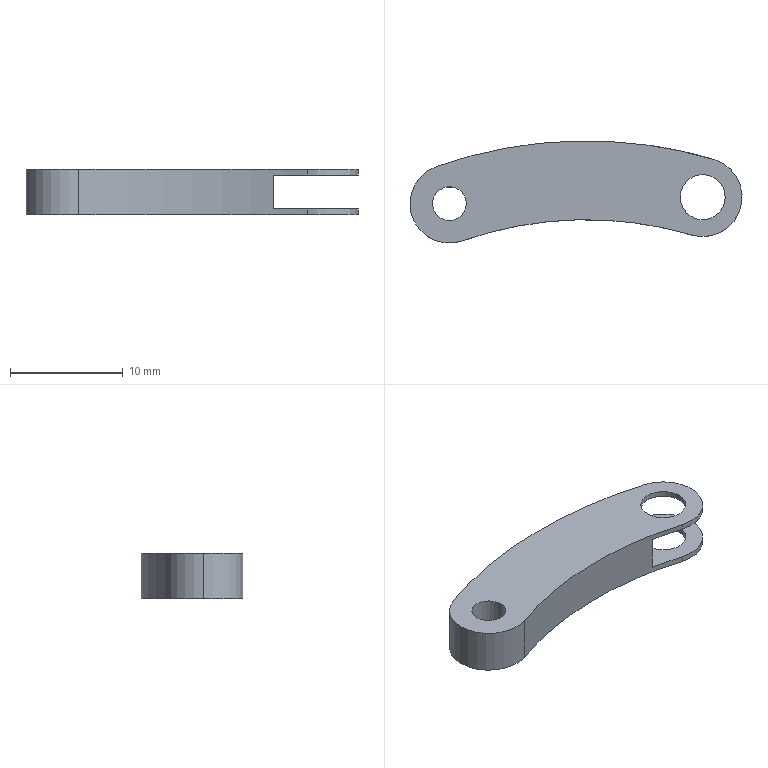Part | SolidWorks | features Extrusion 1, ICE 1, Scale 1 | 1 solid | 17 faces | box 29.5 x 9.079 x 4 mm | volume 609.677 mm3 | cylinder 12 | plane 5 | commonest cylinder face diameters 4 x4 7 x4 3 x2 66 x1 80 x1
STEP:
#1=CARTESIAN_POINT('',(-25.715,-3.325,4.));
#2=VERTEX_POINT('',#1);
#3=CARTESIAN_POINT('',(-22.715,-3.325,4.));
#4=VERTEX_POINT('',#3);
#5=CARTESIAN_POINT('',(-24.215,-3.325,4.));
#6=DIRECTION('',(0.,0.,1.));
#7=DIRECTION('',(1.,0.,0.));
#8=AXIS2_PLACEMENT_3D('',#5,#6,#7);
#9=CIRCLE('',#8,1.5);
#10=EDGE_CURVE('',#2,#4,#9,.T.);
#11=ORIENTED_EDGE('',*,*,#10,.T.);
#12=CARTESIAN_POINT('',(-22.715,-3.325,0.));
#13=VERTEX_POINT('',#12);
#14=CARTESIAN_POINT('',(-22.715,-3.325,4.));
#15=DIRECTION('',(0.,0.,-1.));
#16=VECTOR('',#15,1000.);
#17=LINE('',#14,#16);
#18=EDGE_CURVE('',#4,#13,#17,.T.);
#19=ORIENTED_EDGE('',*,*,#18,.T.);
#20=CARTESIAN_POINT('',(-25.715,-3.325,0.));
#21=VERTEX_POINT('',#20);
#22=CARTESIAN_POINT('',(-24.215,-3.325,0.));
#23=DIRECTION('',(0.,0.,1.));
#24=DIRECTION('',(1.,0.,0.));
#25=AXIS2_PLACEMENT_3D('',#22,#23,#24);
#26=CIRCLE('',#25,1.5);
#27=EDGE_CURVE('',#21,#13,#26,.T.);
#28=ORIENTED_EDGE('',*,*,#27,.F.);
#29=CARTESIAN_POINT('',(-25.715,-3.325,4.));
#30=DIRECTION('',(0.,0.,-1.));
#31=VECTOR('',#30,1000.);
#32=LINE('',#29,#31);
#33=EDGE_CURVE('',#2,#21,#32,.T.);
#34=ORIENTED_EDGE('',*,*,#33,.F.);
#35=EDGE_LOOP('',(#11,#19,#28,#34));
#36=FACE_OUTER_BOUND('',#35,.T.);
#37=CARTESIAN_POINT('',(-24.215,-3.325,4.));
#38=DIRECTION('',(0.,0.,-1.));
#39=DIRECTION('',(-1.,0.,0.));
#40=AXIS2_PLACEMENT_3D('',#37,#38,#39);
#41=CYLINDRICAL_SURFACE('',#40,1.5);
#42=ADVANCED_FACE('',(#36),#41,.F.);
#43=CARTESIAN_POINT('',(-27.715,-3.325,4.));
#44=VERTEX_POINT('',#43);
#45=CARTESIAN_POINT('',(-23.05,-6.626,4.));
#46=VERTEX_POINT('',#45);
#47=CARTESIAN_POINT('',(-24.215,-3.325,4.));
#48=DIRECTION('',(0.,0.,1.));
#49=DIRECTION('',(1.,0.,0.));
#50=AXIS2_PLACEMENT_3D('',#47,#48,#49);
#51=CIRCLE('',#50,3.5);
#52=EDGE_CURVE('',#44,#46,#51,.T.);
#53=ORIENTED_EDGE('',*,*,#52,.F.);
#54=CARTESIAN_POINT('',(-27.715,-3.325,0.));
#55=VERTEX_POINT('',#54);
#56=CARTESIAN_POINT('',(-27.715,-3.325,4.));
#57=DIRECTION('',(0.,0.,-1.));
#58=VECTOR('',#57,1000.);
#59=LINE('',#56,#58);
#60=EDGE_CURVE('',#44,#55,#59,.T.);
#61=ORIENTED_EDGE('',*,*,#60,.T.);
#62=CARTESIAN_POINT('',(-23.05,-6.626,0.));
#63=VERTEX_POINT('',#62);
#64=CARTESIAN_POINT('',(-24.215,-3.325,0.));
#65=DIRECTION('',(0.,0.,1.));
#66=DIRECTION('',(1.,0.,0.));
#67=AXIS2_PLACEMENT_3D('',#64,#65,#66);
#68=CIRCLE('',#67,3.5);
#69=EDGE_CURVE('',#55,#63,#68,.T.);
#70=ORIENTED_EDGE('',*,*,#69,.T.);
#71=CARTESIAN_POINT('',(-23.05,-6.626,4.));
#72=DIRECTION('',(0.,0.,-1.));
#73=VECTOR('',#72,1000.);
#74=LINE('',#71,#73);
#75=EDGE_CURVE('',#46,#63,#74,.T.);
#76=ORIENTED_EDGE('',*,*,#75,.F.);
#77=EDGE_LOOP('',(#53,#61,#70,#76));
#78=FACE_OUTER_BOUND('',#77,.T.);
#79=CARTESIAN_POINT('',(-24.215,-3.325,4.));
#80=DIRECTION('',(0.,0.,-1.));
#81=DIRECTION('',(-1.,0.,0.));
#82=AXIS2_PLACEMENT_3D('',#79,#80,#81);
#83=CYLINDRICAL_SURFACE('',#82,3.5);
#84=ADVANCED_FACE('',(#78),#83,.T.);
#85=CARTESIAN_POINT('',(-3.715,-2.747,4.));
#86=VERTEX_POINT('',#85);
#87=CARTESIAN_POINT('',(0.2854,-2.747,4.));
#88=VERTEX_POINT('',#87);
#89=CARTESIAN_POINT('',(-1.715,-2.747,4.));
#90=DIRECTION('',(0.,0.,1.));
#91=DIRECTION('',(1.,0.,0.));
#92=AXIS2_PLACEMENT_3D('',#89,#90,#91);
#93=CIRCLE('',#92,2.);
#94=EDGE_CURVE('',#86,#88,#93,.T.);
#95=ORIENTED_EDGE('',*,*,#94,.T.);
#96=CARTESIAN_POINT('',(0.2854,-2.747,3.5));
#97=VERTEX_POINT('',#96);
#98=CARTESIAN_POINT('',(0.2854,-2.747,4.));
#99=DIRECTION('',(0.,0.,-1.));
#100=VECTOR('',#99,1000.);
#101=LINE('',#98,#100);
#102=EDGE_CURVE('',#88,#97,#101,.T.);
#103=ORIENTED_EDGE('',*,*,#102,.T.);
#104=CARTESIAN_POINT('',(-3.715,-2.747,3.5));
#105=VERTEX_POINT('',#104);
#106=CARTESIAN_POINT('',(-1.715,-2.747,3.5));
#107=DIRECTION('',(0.,0.,-1.));
#108=DIRECTION('',(-1.,0.,0.));
#109=AXIS2_PLACEMENT_3D('',#106,#107,#108);
#110=CIRCLE('',#109,2.);
#111=EDGE_CURVE('',#97,#105,#110,.T.);
#112=ORIENTED_EDGE('',*,*,#111,.T.);
#113=CARTESIAN_POINT('',(-3.715,-2.747,4.));
#114=DIRECTION('',(0.,0.,-1.));
#115=VECTOR('',#114,1000.);
#116=LINE('',#113,#115);
#117=EDGE_CURVE('',#86,#105,#116,.T.);
#118=ORIENTED_EDGE('',*,*,#117,.F.);
#119=EDGE_LOOP('',(#95,#103,#112,#118));
#120=FACE_OUTER_BOUND('',#119,.T.);
#121=CARTESIAN_POINT('',(-1.715,-2.747,4.));
#122=DIRECTION('',(0.,0.,-1.));
#123=DIRECTION('',(-1.,0.,0.));
#124=AXIS2_PLACEMENT_3D('',#121,#122,#123);
#125=CYLINDRICAL_SURFACE('',#124,2.);
#126=ADVANCED_FACE('',(#120),#125,.F.);
#127=CARTESIAN_POINT('',(-3.715,-2.747,0.5));
#128=VERTEX_POINT('',#127);
#129=CARTESIAN_POINT('',(0.2854,-2.747,0.5));
#130=VERTEX_POINT('',#129);
#131=CARTESIAN_POINT('',(-1.715,-2.747,0.5));
#132=DIRECTION('',(0.,0.,1.));
#133=DIRECTION('',(1.,0.,0.));
#134=AXIS2_PLACEMENT_3D('',#131,#132,#133);
#135=CIRCLE('',#134,2.);
#136=EDGE_CURVE('',#128,#130,#135,.T.);
#137=ORIENTED_EDGE('',*,*,#136,.T.);
#138=CARTESIAN_POINT('',(0.2854,-2.747,0.));
#139=VERTEX_POINT('',#138);
#140=CARTESIAN_POINT('',(0.2854,-2.747,4.));
#141=DIRECTION('',(0.,0.,-1.));
#142=VECTOR('',#141,1000.);
#143=LINE('',#140,#142);
#144=EDGE_CURVE('',#130,#139,#143,.T.);
#145=ORIENTED_EDGE('',*,*,#144,.T.);
#146=CARTESIAN_POINT('',(-3.715,-2.747,0.));
#147=VERTEX_POINT('',#146);
#148=CARTESIAN_POINT('',(-1.715,-2.747,0.));
#149=DIRECTION('',(0.,0.,1.));
#150=DIRECTION('',(1.,0.,0.));
#151=AXIS2_PLACEMENT_3D('',#148,#149,#150);
#152=CIRCLE('',#151,2.);
#153=EDGE_CURVE('',#147,#139,#152,.T.);
#154=ORIENTED_EDGE('',*,*,#153,.F.);
#155=CARTESIAN_POINT('',(-3.715,-2.747,4.));
#156=DIRECTION('',(0.,0.,-1.));
#157=VECTOR('',#156,1000.);
#158=LINE('',#155,#157);
#159=EDGE_CURVE('',#128,#147,#158,.T.);
#160=ORIENTED_EDGE('',*,*,#159,.F.);
#161=EDGE_LOOP('',(#137,#145,#154,#160));
#162=FACE_OUTER_BOUND('',#161,.T.);
#163=CARTESIAN_POINT('',(-1.715,-2.747,4.));
#164=DIRECTION('',(0.,0.,-1.));
#165=DIRECTION('',(-1.,0.,0.));
#166=AXIS2_PLACEMENT_3D('',#163,#164,#165);
#167=CYLINDRICAL_SURFACE('',#166,2.);
#168=ADVANCED_FACE('',(#162),#167,.F.);
#169=CARTESIAN_POINT('',(-5.715,-5.364,0.5));
#170=VERTEX_POINT('',#169);
#171=CARTESIAN_POINT('',(-2.708,-6.103,0.5));
#172=VERTEX_POINT('',#171);
#173=CARTESIAN_POINT('',(-12.072,-37.746,0.5));
#174=DIRECTION('',(0.,0.,-1.));
#175=DIRECTION('',(1.,0.,0.));
#176=AXIS2_PLACEMENT_3D('',#173,#174,#175);
#177=CIRCLE('',#176,33.);
#178=EDGE_CURVE('',#170,#172,#177,.T.);
#179=ORIENTED_EDGE('',*,*,#178,.F.);
#180=CARTESIAN_POINT('',(-5.715,-5.364,3.5));
#181=VERTEX_POINT('',#180);
#182=CARTESIAN_POINT('',(-5.715,-5.364,4.));
#183=DIRECTION('',(0.,0.,-1.));
#184=VECTOR('',#183,1000.);
#185=LINE('',#182,#184);
#186=EDGE_CURVE('',#181,#170,#185,.T.);
#187=ORIENTED_EDGE('',*,*,#186,.F.);
#188=CARTESIAN_POINT('',(-2.708,-6.103,3.5));
#189=VERTEX_POINT('',#188);
#190=CARTESIAN_POINT('',(-12.072,-37.746,3.5));
#191=DIRECTION('',(0.,0.,1.));
#192=DIRECTION('',(-1.,0.,0.));
#193=AXIS2_PLACEMENT_3D('',#190,#191,#192);
#194=CIRCLE('',#193,33.);
#195=EDGE_CURVE('',#189,#181,#194,.T.);
#196=ORIENTED_EDGE('',*,*,#195,.F.);
#197=CARTESIAN_POINT('',(-2.708,-6.103,4.));
#198=VERTEX_POINT('',#197);
#199=CARTESIAN_POINT('',(-2.708,-6.103,4.));
#200=DIRECTION('',(0.,0.,-1.));
#201=VECTOR('',#200,1000.);
#202=LINE('',#199,#201);
#203=EDGE_CURVE('',#198,#189,#202,.T.);
#204=ORIENTED_EDGE('',*,*,#203,.F.);
#205=CARTESIAN_POINT('',(-12.072,-37.746,4.));
#206=DIRECTION('',(0.,0.,-1.));
#207=DIRECTION('',(-1.,0.,0.));
#208=AXIS2_PLACEMENT_3D('',#205,#206,#207);
#209=CIRCLE('',#208,33.);
#210=EDGE_CURVE('',#46,#198,#209,.T.);
#211=ORIENTED_EDGE('',*,*,#210,.F.);
#212=ORIENTED_EDGE('',*,*,#75,.T.);
#213=CARTESIAN_POINT('',(-2.708,-6.103,0.));
#214=VERTEX_POINT('',#213);
#215=CARTESIAN_POINT('',(-12.072,-37.746,0.));
#216=DIRECTION('',(0.,0.,-1.));
#217=DIRECTION('',(-1.,0.,0.));
#218=AXIS2_PLACEMENT_3D('',#215,#216,#217);
#219=CIRCLE('',#218,33.);
#220=EDGE_CURVE('',#63,#214,#219,.T.);
#221=ORIENTED_EDGE('',*,*,#220,.T.);
#222=CARTESIAN_POINT('',(-2.708,-6.103,4.));
#223=DIRECTION('',(0.,0.,-1.));
#224=VECTOR('',#223,1000.);
#225=LINE('',#222,#224);
#226=EDGE_CURVE('',#172,#214,#225,.T.);
#227=ORIENTED_EDGE('',*,*,#226,.F.);
#228=EDGE_LOOP('',(#179,#187,#196,#204,#211,#212,#221,#227));
#229=FACE_OUTER_BOUND('',#228,.T.);
#230=CARTESIAN_POINT('',(-12.072,-37.746,4.));
#231=DIRECTION('',(0.,0.,-1.));
#232=DIRECTION('',(-1.,0.,0.));
#233=AXIS2_PLACEMENT_3D('',#230,#231,#232);
#234=CYLINDRICAL_SURFACE('',#233,33.);
#235=ADVANCED_FACE('',(#229),#234,.F.);
#236=CARTESIAN_POINT('',(-0.7214,0.6095,0.5));
#237=VERTEX_POINT('',#236);
#238=CARTESIAN_POINT('',(-1.715,-2.747,0.5));
#239=DIRECTION('',(0.,0.,1.));
#240=DIRECTION('',(1.,0.,0.));
#241=AXIS2_PLACEMENT_3D('',#238,#239,#240);
#242=CIRCLE('',#241,3.5);
#243=EDGE_CURVE('',#172,#237,#242,.T.);
#244=ORIENTED_EDGE('',*,*,#243,.F.);
#245=ORIENTED_EDGE('',*,*,#226,.T.);
#246=CARTESIAN_POINT('',(-0.7214,0.6095,0.));
#247=VERTEX_POINT('',#246);
#248=CARTESIAN_POINT('',(-1.715,-2.747,0.));
#249=DIRECTION('',(0.,0.,1.));
#250=DIRECTION('',(1.,0.,0.));
#251=AXIS2_PLACEMENT_3D('',#248,#249,#250);
#252=CIRCLE('',#251,3.5);
#253=EDGE_CURVE('',#214,#247,#252,.T.);
#254=ORIENTED_EDGE('',*,*,#253,.T.);
#255=CARTESIAN_POINT('',(-0.7214,0.6095,4.));
#256=DIRECTION('',(0.,0.,-1.));
#257=VECTOR('',#256,1000.);
#258=LINE('',#255,#257);
#259=EDGE_CURVE('',#237,#247,#258,.T.);
#260=ORIENTED_EDGE('',*,*,#259,.F.);
#261=EDGE_LOOP('',(#244,#245,#254,#260));
#262=FACE_OUTER_BOUND('',#261,.T.);
#263=CARTESIAN_POINT('',(-1.715,-2.747,4.));
#264=DIRECTION('',(0.,0.,-1.));
#265=DIRECTION('',(-1.,0.,0.));
#266=AXIS2_PLACEMENT_3D('',#263,#264,#265);
#267=CYLINDRICAL_SURFACE('',#266,3.5);
#268=ADVANCED_FACE('',(#262),#267,.T.);
#269=CARTESIAN_POINT('',(-0.7214,0.6095,3.5));
#270=VERTEX_POINT('',#269);
#271=CARTESIAN_POINT('',(-1.715,-2.747,3.5));
#272=DIRECTION('',(0.,0.,-1.));
#273=DIRECTION('',(-1.,0.,0.));
#274=AXIS2_PLACEMENT_3D('',#271,#272,#273);
#275=CIRCLE('',#274,3.5);
#276=EDGE_CURVE('',#270,#189,#275,.T.);
#277=ORIENTED_EDGE('',*,*,#276,.F.);
#278=CARTESIAN_POINT('',(-0.7214,0.6095,4.));
#279=VERTEX_POINT('',#278);
#280=CARTESIAN_POINT('',(-0.7214,0.6095,4.));
#281=DIRECTION('',(0.,0.,-1.));
#282=VECTOR('',#281,1000.);
#283=LINE('',#280,#282);
#284=EDGE_CURVE('',#279,#270,#283,.T.);
#285=ORIENTED_EDGE('',*,*,#284,.F.);
#286=CARTESIAN_POINT('',(-1.715,-2.747,4.));
#287=DIRECTION('',(0.,0.,1.));
#288=DIRECTION('',(1.,0.,0.));
#289=AXIS2_PLACEMENT_3D('',#286,#287,#288);
#290=CIRCLE('',#289,3.5);
#291=EDGE_CURVE('',#198,#279,#290,.T.);
#292=ORIENTED_EDGE('',*,*,#291,.F.);
#293=ORIENTED_EDGE('',*,*,#203,.T.);
#294=EDGE_LOOP('',(#277,#285,#292,#293));
#295=FACE_OUTER_BOUND('',#294,.T.);
#296=CARTESIAN_POINT('',(-1.715,-2.747,4.));
#297=DIRECTION('',(0.,0.,-1.));
#298=DIRECTION('',(-1.,0.,0.));
#299=AXIS2_PLACEMENT_3D('',#296,#297,#298);
#300=CYLINDRICAL_SURFACE('',#299,3.5);
#301=ADVANCED_FACE('',(#295),#300,.T.);
#302=CARTESIAN_POINT('',(-5.715,1.745,0.5));
#303=VERTEX_POINT('',#302);
#304=CARTESIAN_POINT('',(-12.072,-37.746,0.5));
#305=DIRECTION('',(0.,0.,1.));
#306=DIRECTION('',(1.,0.,0.));
#307=AXIS2_PLACEMENT_3D('',#304,#305,#306);
#308=CIRCLE('',#307,40.);
#309=EDGE_CURVE('',#237,#303,#308,.T.);
#310=ORIENTED_EDGE('',*,*,#309,.F.);
#311=ORIENTED_EDGE('',*,*,#259,.T.);
#312=CARTESIAN_POINT('',(-25.379,-0.0244,0.));
#313=VERTEX_POINT('',#312);
#314=CARTESIAN_POINT('',(-12.072,-37.746,0.));
#315=DIRECTION('',(0.,0.,1.));
#316=DIRECTION('',(-1.,0.,0.));
#317=AXIS2_PLACEMENT_3D('',#314,#315,#316);
#318=CIRCLE('',#317,40.);
#319=EDGE_CURVE('',#247,#313,#318,.T.);
#320=ORIENTED_EDGE('',*,*,#319,.T.);
#321=CARTESIAN_POINT('',(-25.379,-0.0244,4.));
#322=VERTEX_POINT('',#321);
#323=CARTESIAN_POINT('',(-25.379,-0.0244,4.));
#324=DIRECTION('',(0.,0.,-1.));
#325=VECTOR('',#324,1000.);
#326=LINE('',#323,#325);
#327=EDGE_CURVE('',#322,#313,#326,.T.);
#328=ORIENTED_EDGE('',*,*,#327,.F.);
#329=CARTESIAN_POINT('',(-12.072,-37.746,4.));
#330=DIRECTION('',(0.,0.,1.));
#331=DIRECTION('',(-1.,0.,0.));
#332=AXIS2_PLACEMENT_3D('',#329,#330,#331);
#333=CIRCLE('',#332,40.);
#334=EDGE_CURVE('',#279,#322,#333,.T.);
#335=ORIENTED_EDGE('',*,*,#334,.F.);
#336=ORIENTED_EDGE('',*,*,#284,.T.);
#337=CARTESIAN_POINT('',(-5.715,1.745,3.5));
#338=VERTEX_POINT('',#337);
#339=CARTESIAN_POINT('',(-12.072,-37.746,3.5));
#340=DIRECTION('',(0.,0.,-1.));
#341=DIRECTION('',(-1.,0.,0.));
#342=AXIS2_PLACEMENT_3D('',#339,#340,#341);
#343=CIRCLE('',#342,40.);
#344=EDGE_CURVE('',#338,#270,#343,.T.);
#345=ORIENTED_EDGE('',*,*,#344,.F.);
#346=CARTESIAN_POINT('',(-5.715,1.745,4.));
#347=DIRECTION('',(0.,0.,1.));
#348=VECTOR('',#347,1000.);
#349=LINE('',#346,#348);
#350=EDGE_CURVE('',#303,#338,#349,.T.);
#351=ORIENTED_EDGE('',*,*,#350,.F.);
#352=EDGE_LOOP('',(#310,#311,#320,#328,#335,#336,#345,#351));
#353=FACE_OUTER_BOUND('',#352,.T.);
#354=CARTESIAN_POINT('',(-12.072,-37.746,4.));
#355=DIRECTION('',(0.,0.,-1.));
#356=DIRECTION('',(-1.,0.,0.));
#357=AXIS2_PLACEMENT_3D('',#354,#355,#356);
#358=CYLINDRICAL_SURFACE('',#357,40.);
#359=ADVANCED_FACE('',(#353),#358,.T.);
#360=ORIENTED_EDGE('',*,*,#144,.F.);
#361=CARTESIAN_POINT('',(-1.715,-2.747,0.5));
#362=DIRECTION('',(0.,0.,1.));
#363=DIRECTION('',(1.,0.,0.));
#364=AXIS2_PLACEMENT_3D('',#361,#362,#363);
#365=CIRCLE('',#364,2.);
#366=EDGE_CURVE('',#130,#128,#365,.T.);
#367=ORIENTED_EDGE('',*,*,#366,.T.);
#368=ORIENTED_EDGE('',*,*,#159,.T.);
#369=CARTESIAN_POINT('',(-1.715,-2.747,0.));
#370=DIRECTION('',(0.,0.,1.));
#371=DIRECTION('',(1.,0.,0.));
#372=AXIS2_PLACEMENT_3D('',#369,#370,#371);
#373=CIRCLE('',#372,2.);
#374=EDGE_CURVE('',#139,#147,#373,.T.);
#375=ORIENTED_EDGE('',*,*,#374,.F.);
#376=EDGE_LOOP('',(#360,#367,#368,#375));
#377=FACE_OUTER_BOUND('',#376,.T.);
#378=CARTESIAN_POINT('',(-1.715,-2.747,4.));
#379=DIRECTION('',(0.,0.,-1.));
#380=DIRECTION('',(-1.,0.,0.));
#381=AXIS2_PLACEMENT_3D('',#378,#379,#380);
#382=CYLINDRICAL_SURFACE('',#381,2.);
#383=ADVANCED_FACE('',(#377),#382,.F.);
#384=ORIENTED_EDGE('',*,*,#102,.F.);
#385=CARTESIAN_POINT('',(-1.715,-2.747,4.));
#386=DIRECTION('',(0.,0.,1.));
#387=DIRECTION('',(1.,0.,0.));
#388=AXIS2_PLACEMENT_3D('',#385,#386,#387);
#389=CIRCLE('',#388,2.);
#390=EDGE_CURVE('',#88,#86,#389,.T.);
#391=ORIENTED_EDGE('',*,*,#390,.T.);
#392=ORIENTED_EDGE('',*,*,#117,.T.);
#393=CARTESIAN_POINT('',(-1.715,-2.747,3.5));
#394=DIRECTION('',(0.,0.,-1.));
#395=DIRECTION('',(-1.,0.,0.));
#396=AXIS2_PLACEMENT_3D('',#393,#394,#395);
#397=CIRCLE('',#396,2.);
#398=EDGE_CURVE('',#105,#97,#397,.T.);
#399=ORIENTED_EDGE('',*,*,#398,.T.);
#400=EDGE_LOOP('',(#384,#391,#392,#399));
#401=FACE_OUTER_BOUND('',#400,.T.);
#402=CARTESIAN_POINT('',(-1.715,-2.747,4.));
#403=DIRECTION('',(0.,0.,-1.));
#404=DIRECTION('',(-1.,0.,0.));
#405=AXIS2_PLACEMENT_3D('',#402,#403,#404);
#406=CYLINDRICAL_SURFACE('',#405,2.);
#407=ADVANCED_FACE('',(#401),#406,.F.);
#408=ORIENTED_EDGE('',*,*,#10,.F.);
#409=CARTESIAN_POINT('',(-24.215,-3.325,4.));
#410=DIRECTION('',(0.,0.,1.));
#411=DIRECTION('',(1.,0.,0.));
#412=AXIS2_PLACEMENT_3D('',#409,#410,#411);
#413=CIRCLE('',#412,1.5);
#414=EDGE_CURVE('',#4,#2,#413,.T.);
#415=ORIENTED_EDGE('',*,*,#414,.F.);
#416=EDGE_LOOP('',(#408,#415));
#417=FACE_BOUND('',#416,.T.);
#418=CARTESIAN_POINT('',(-24.215,-3.325,4.));
#419=DIRECTION('',(0.,0.,1.));
#420=DIRECTION('',(1.,0.,0.));
#421=AXIS2_PLACEMENT_3D('',#418,#419,#420);
#422=CIRCLE('',#421,3.5);
#423=EDGE_CURVE('',#322,#44,#422,.T.);
#424=ORIENTED_EDGE('',*,*,#423,.T.);
#425=ORIENTED_EDGE('',*,*,#52,.T.);
#426=ORIENTED_EDGE('',*,*,#210,.T.);
#427=ORIENTED_EDGE('',*,*,#291,.T.);
#428=ORIENTED_EDGE('',*,*,#334,.T.);
#429=EDGE_LOOP('',(#424,#425,#426,#427,#428));
#430=FACE_OUTER_BOUND('',#429,.T.);
#431=ORIENTED_EDGE('',*,*,#94,.F.);
#432=ORIENTED_EDGE('',*,*,#390,.F.);
#433=EDGE_LOOP('',(#431,#432));
#434=FACE_BOUND('',#433,.T.);
#435=CARTESIAN_POINT('',(-18.143,-20.536,4.));
#436=DIRECTION('',(0.,0.,1.));
#437=DIRECTION('',(1.,0.,0.));
#438=AXIS2_PLACEMENT_3D('',#435,#436,#437);
#439=PLANE('',#438);
#440=ADVANCED_FACE('',(#417,#430,#434),#439,.T.);
#441=CARTESIAN_POINT('',(-24.215,-3.325,0.));
#442=DIRECTION('',(0.,0.,1.));
#443=DIRECTION('',(1.,0.,0.));
#444=AXIS2_PLACEMENT_3D('',#441,#442,#443);
#445=CIRCLE('',#444,3.5);
#446=EDGE_CURVE('',#313,#55,#445,.T.);
#447=ORIENTED_EDGE('',*,*,#446,.F.);
#448=ORIENTED_EDGE('',*,*,#319,.F.);
#449=ORIENTED_EDGE('',*,*,#253,.F.);
#450=ORIENTED_EDGE('',*,*,#220,.F.);
#451=ORIENTED_EDGE('',*,*,#69,.F.);
#452=EDGE_LOOP('',(#447,#448,#449,#450,#451));
#453=FACE_OUTER_BOUND('',#452,.T.);
#454=ORIENTED_EDGE('',*,*,#27,.T.);
#455=CARTESIAN_POINT('',(-24.215,-3.325,0.));
#456=DIRECTION('',(0.,0.,1.));
#457=DIRECTION('',(1.,0.,0.));
#458=AXIS2_PLACEMENT_3D('',#455,#456,#457);
#459=CIRCLE('',#458,1.5);
#460=EDGE_CURVE('',#13,#21,#459,.T.);
#461=ORIENTED_EDGE('',*,*,#460,.T.);
#462=EDGE_LOOP('',(#454,#461));
#463=FACE_BOUND('',#462,.T.);
#464=ORIENTED_EDGE('',*,*,#153,.T.);
#465=ORIENTED_EDGE('',*,*,#374,.T.);
#466=EDGE_LOOP('',(#464,#465));
#467=FACE_BOUND('',#466,.T.);
#468=CARTESIAN_POINT('',(-18.143,-20.536,0.));
#469=DIRECTION('',(0.,0.,1.));
#470=DIRECTION('',(1.,0.,0.));
#471=AXIS2_PLACEMENT_3D('',#468,#469,#470);
#472=PLANE('',#471);
#473=ADVANCED_FACE('',(#453,#463,#467),#472,.F.);
#474=ORIENTED_EDGE('',*,*,#60,.F.);
#475=ORIENTED_EDGE('',*,*,#423,.F.);
#476=ORIENTED_EDGE('',*,*,#327,.T.);
#477=ORIENTED_EDGE('',*,*,#446,.T.);
#478=EDGE_LOOP('',(#474,#475,#476,#477));
#479=FACE_OUTER_BOUND('',#478,.T.);
#480=CARTESIAN_POINT('',(-24.215,-3.325,4.));
#481=DIRECTION('',(0.,0.,-1.));
#482=DIRECTION('',(-1.,0.,0.));
#483=AXIS2_PLACEMENT_3D('',#480,#481,#482);
#484=CYLINDRICAL_SURFACE('',#483,3.5);
#485=ADVANCED_FACE('',(#479),#484,.T.);
#486=ORIENTED_EDGE('',*,*,#18,.F.);
#487=ORIENTED_EDGE('',*,*,#414,.T.);
#488=ORIENTED_EDGE('',*,*,#33,.T.);
#489=ORIENTED_EDGE('',*,*,#460,.F.);
#490=EDGE_LOOP('',(#486,#487,#488,#489));
#491=FACE_OUTER_BOUND('',#490,.T.);
#492=CARTESIAN_POINT('',(-24.215,-3.325,4.));
#493=DIRECTION('',(0.,0.,-1.));
#494=DIRECTION('',(-1.,0.,0.));
#495=AXIS2_PLACEMENT_3D('',#492,#493,#494);
#496=CYLINDRICAL_SURFACE('',#495,1.5);
#497=ADVANCED_FACE('',(#491),#496,.F.);
#498=ORIENTED_EDGE('',*,*,#186,.T.);
#499=CARTESIAN_POINT('',(-5.715,4.,0.5));
#500=DIRECTION('',(0.,-1.,0.));
#501=VECTOR('',#500,1000.);
#502=LINE('',#499,#501);
#503=EDGE_CURVE('',#303,#170,#502,.T.);
#504=ORIENTED_EDGE('',*,*,#503,.F.);
#505=ORIENTED_EDGE('',*,*,#350,.T.);
#506=CARTESIAN_POINT('',(-5.715,4.,3.5));
#507=DIRECTION('',(0.,-1.,0.));
#508=VECTOR('',#507,1000.);
#509=LINE('',#506,#508);
#510=EDGE_CURVE('',#338,#181,#509,.T.);
#511=ORIENTED_EDGE('',*,*,#510,.T.);
#512=EDGE_LOOP('',(#498,#504,#505,#511));
#513=FACE_OUTER_BOUND('',#512,.T.);
#514=CARTESIAN_POINT('',(-5.715,4.,0.5));
#515=DIRECTION('',(1.,0.,0.));
#516=DIRECTION('',(0.,0.,-1.));
#517=AXIS2_PLACEMENT_3D('',#514,#515,#516);
#518=PLANE('',#517);
#519=ADVANCED_FACE('',(#513),#518,.T.);
#520=ORIENTED_EDGE('',*,*,#136,.F.);
#521=ORIENTED_EDGE('',*,*,#366,.F.);
#522=EDGE_LOOP('',(#520,#521));
#523=FACE_BOUND('',#522,.T.);
#524=ORIENTED_EDGE('',*,*,#178,.T.);
#525=ORIENTED_EDGE('',*,*,#243,.T.);
#526=ORIENTED_EDGE('',*,*,#309,.T.);
#527=ORIENTED_EDGE('',*,*,#503,.T.);
#528=EDGE_LOOP('',(#524,#525,#526,#527));
#529=FACE_OUTER_BOUND('',#528,.T.);
#530=CARTESIAN_POINT('',(-5.715,4.,0.5));
#531=DIRECTION('',(0.,0.,1.));
#532=DIRECTION('',(1.,0.,0.));
#533=AXIS2_PLACEMENT_3D('',#530,#531,#532);
#534=PLANE('',#533);
#535=ADVANCED_FACE('',(#523,#529),#534,.T.);
#536=ORIENTED_EDGE('',*,*,#398,.F.);
#537=ORIENTED_EDGE('',*,*,#111,.F.);
#538=EDGE_LOOP('',(#536,#537));
#539=FACE_BOUND('',#538,.T.);
#540=ORIENTED_EDGE('',*,*,#195,.T.);
#541=ORIENTED_EDGE('',*,*,#510,.F.);
#542=ORIENTED_EDGE('',*,*,#344,.T.);
#543=ORIENTED_EDGE('',*,*,#276,.T.);
#544=EDGE_LOOP('',(#540,#541,#542,#543));
#545=FACE_OUTER_BOUND('',#544,.T.);
#546=CARTESIAN_POINT('',(-5.715,4.,3.5));
#547=DIRECTION('',(0.,0.,-1.));
#548=DIRECTION('',(-1.,0.,0.));
#549=AXIS2_PLACEMENT_3D('',#546,#547,#548);
#550=PLANE('',#549);
#551=ADVANCED_FACE('',(#539,#545),#550,.T.);
#552=CLOSED_SHELL('',(#42,#84,#126,#168,#235,#268,#301,#359,#383,#407,#440,#473,#485,#497,#519,#535,#551));
#553=MANIFOLD_SOLID_BREP('',#552);
#554=CARTESIAN_POINT('',(0.,0.,0.));
#555=DIRECTION('',(0.,0.,1.));
#556=DIRECTION('',(1.,0.,0.));
#557=AXIS2_PLACEMENT_3D('',#554,#555,#556);
#558=(LENGTH_UNIT()NAMED_UNIT(*)SI_UNIT(.MILLI.,.METRE.));
#559=UNCERTAINTY_MEASURE_WITH_UNIT(LENGTH_MEASURE(0.00001),#558,'','');
#560=(NAMED_UNIT(*)PLANE_ANGLE_UNIT()SI_UNIT($,.RADIAN.));
#561=(NAMED_UNIT(*)SI_UNIT($,.STERADIAN.)SOLID_ANGLE_UNIT());
#562=(GEOMETRIC_REPRESENTATION_CONTEXT(3)GLOBAL_UNCERTAINTY_ASSIGNED_CONTEXT((#559))GLOBAL_UNIT_ASSIGNED_CONTEXT((#558,#560,#561))REPRESENTATION_CONTEXT('',''));
#563=ADVANCED_BREP_SHAPE_REPRESENTATION('',(#553,#557),#562);